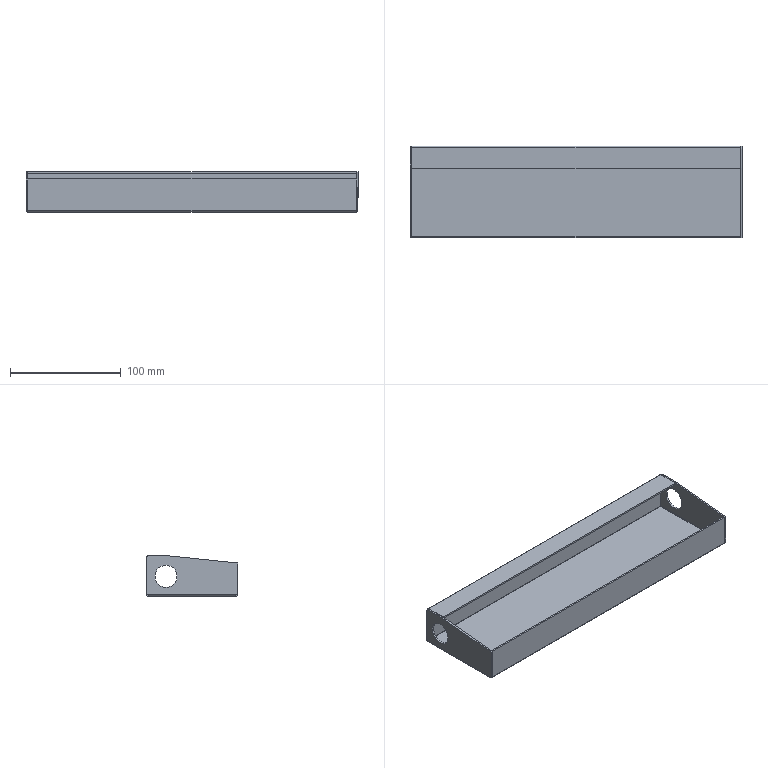Part | SolidWorks | features EdgeFlange 4, Fillet 2, CornerFeat 1, FlatPattern 1, ICE 1, SMBaseFlange 1, SheetMetal 1 | 1 solid | 62 faces | box 300 x 83 x 36.5 mm | volume 80291 mm3 | plane 46 | cylinder 16 | commonest cylinder face diameters 0.5 x5 3.5 x5 20 x4 6 x2